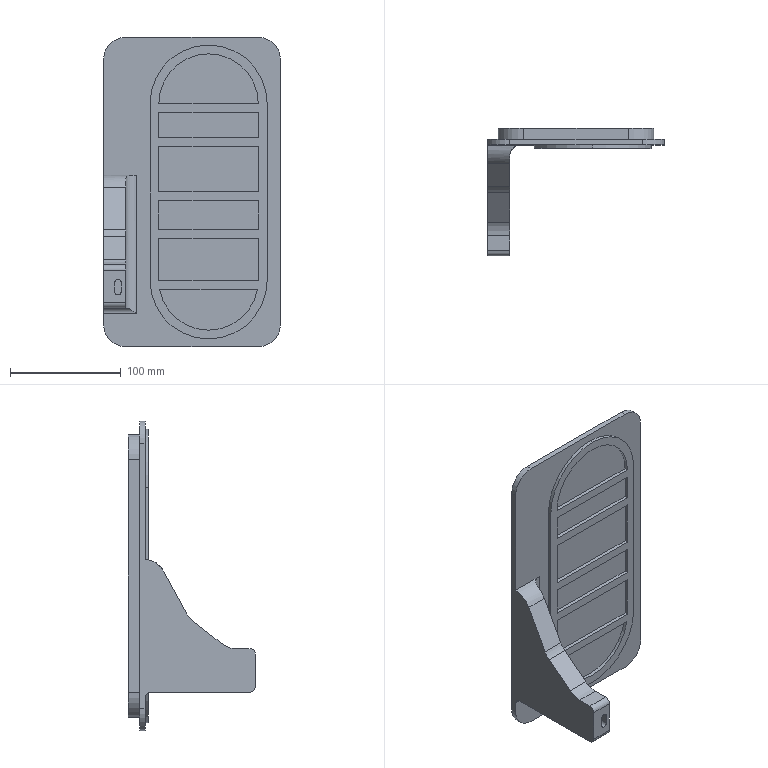Part | SolidWorks | features Fillet 5, ICE 4, BossThin 2, Chamfer 1, Extrusion 1 | 1 solid | 111 faces | box 160 x 115 x 280 mm | volume 478660 mm3 | plane 79 | cylinder 32 | commonest cylinder face diameters 34 x8 40 x7 46 x4 6 x3 10 x3 90 x3